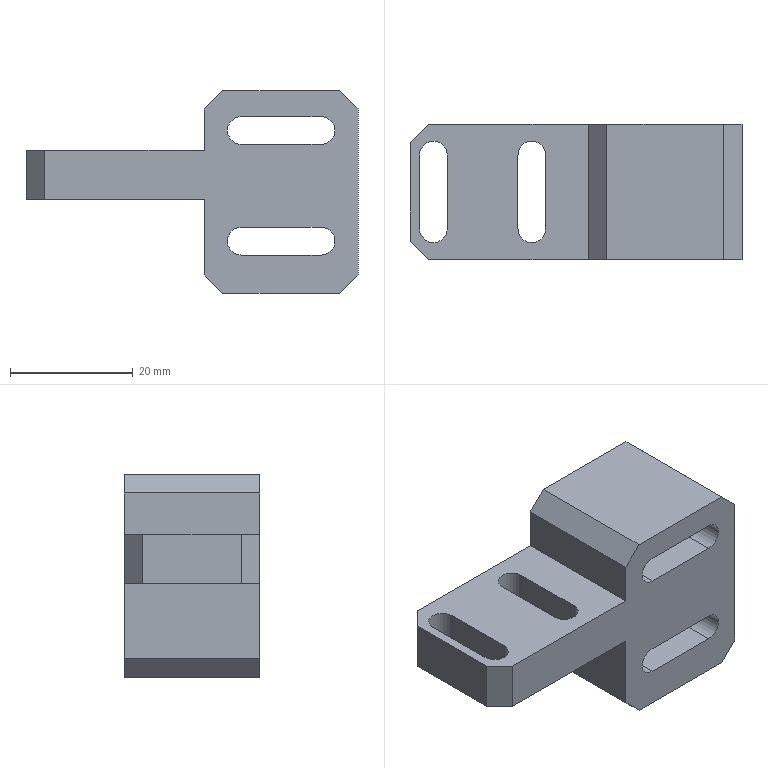Part | STEP file | 0-19 Finger cylinder fixed plate | 1 solid | 32 faces | box 54 x 22 x 33 mm | volume 18394 mm3 | plane 24 | cylinder 8 | commonest cylinder face diameters 4.5 x8